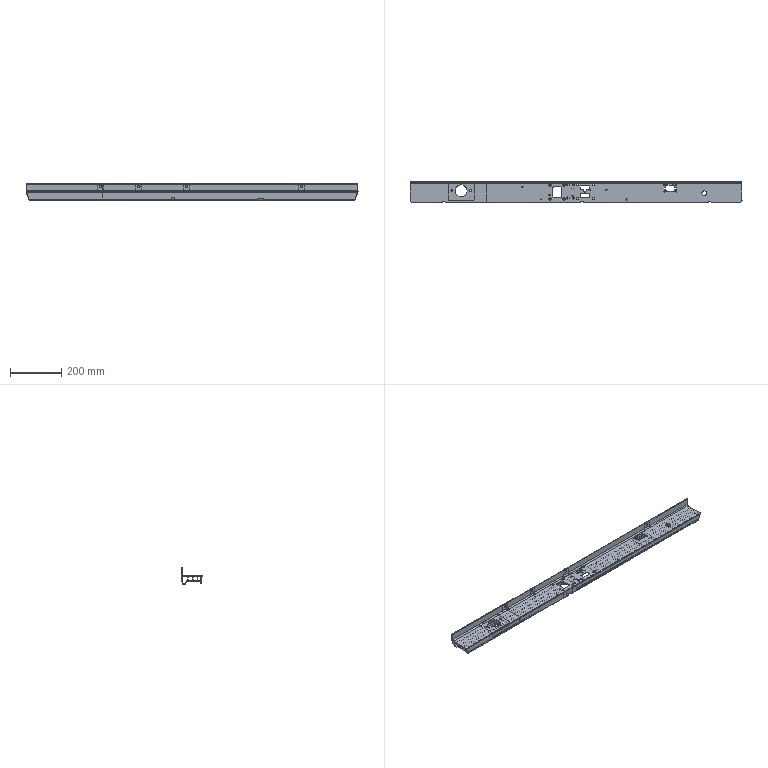NC program | NX | posted with a generic post | part box 1301 x 81.1 x 63 mm
Whole program:
N10 G17 G21 G94 G90
(HOLE_MILLING_1_COPY_2 , TOOL : D6)
N12 T06 M6
N14 G54
N16 G17 G0 G90 X0. Y-10. B0. C0. S6000 M3
N18 G43 Z30. H6
N20 Z0.2
N22 G94 G3 X-0.688 Y-9.313 R0.688 F1400.
N24 X-1.375 Y-10. R0.688
N26 X-1.375 Y-10. Z-0.3 I1.375 J0.
N28 X-1.375 Y-10. Z-0.8 I1.375 J0.
N30 X-1.375 Y-10. Z-1.3 I1.375 J0.
N32 X-1.375 Y-10. Z-1.8 I1.375 J0.
N34 X-1.375 Y-10. Z-2.3 I1.375 J0.
N36 X-1.375 Y-10. Z-2.8 I1.375 J0.
N38 X-1.375 Y-10. Z-3.3 I1.375 J0.
N40 X-1.375 Y-10. Z-3.8 I1.375 J0.
N42 X0. Y-11.375 R1.375
N44 X-1.375 Y-10. R-1.375
N46 X-0.688 Y-10.688 R0.688
N48 X0. Y-10. R0.688
N50 G0 Z30.
N52 X448.999
N54 Z0.2
N56 G3 X448.312 Y-9.313 R0.688
N58 X447.624 Y-10. R0.688
N60 X447.624 Y-10. Z-0.3 I1.375 J0.
N62 X447.624 Y-10. Z-0.8 I1.375 J0.
N64 X447.624 Y-10. Z-1.3 I1.375 J0.
N66 X447.624 Y-10. Z-1.8 I1.375 J0.
N68 X447.624 Y-10. Z-2.3 I1.375 J0.
N70 X447.624 Y-10. Z-2.8 I1.375 J0.
N72 X447.624 Y-10. Z-3.3 I1.375 J0.
N74 X447.624 Y-10. Z-3.8 I1.375 J0.
N76 X448.999 Y-11.375 R1.375
N78 X447.624 Y-10. R-1.375
N80 X448.312 Y-10.688 R0.688
N82 X448.999 Y-10. R0.688
N84 G0 Z30.
N86 X635.999
N88 Z0.2
N90 G3 X635.312 Y-9.313 R0.688
N92 X634.624 Y-10. R0.688
N94 X634.624 Y-10. Z-0.3 I1.375 J0.
N96 X634.624 Y-10. Z-0.8 I1.375 J0.
N98 X634.624 Y-10. Z-1.3 I1.375 J0.
N100 X634.624 Y-10. Z-1.8 I1.375 J0.
N102 X634.624 Y-10. Z-2.3 I1.375 J0.
N104 X634.624 Y-10. Z-2.8 I1.375 J0.
N106 X634.624 Y-10. Z-3.3 I1.375 J0.
N108 X634.624 Y-10. Z-3.8 I1.375 J0.
N110 X635.999 Y-11.375 R1.375
N112 X634.624 Y-10. R-1.375
N114 X635.312 Y-10.688 R0.688
N116 X635.999 Y-10. R0.688
N118 G0 Z30.
N120 X785.999
N122 Z0.2
N124 G3 X785.312 Y-9.313 R0.688
N126 X784.624 Y-10. R0.688
N128 X784.624 Y-10. Z-0.3 I1.375 J0.
N130 X784.624 Y-10. Z-0.8 I1.375 J0.
N132 X784.624 Y-10. Z-1.3 I1.375 J0.
N134 X784.624 Y-10. Z-1.8 I1.375 J0.
N136 X784.624 Y-10. Z-2.3 I1.375 J0.
N138 X784.624 Y-10. Z-2.8 I1.375 J0.
N140 X784.624 Y-10. Z-3.3 I1.375 J0.
N142 X784.624 Y-10. Z-3.8 I1.375 J0.
N144 X785.999 Y-11.375 R1.375
N146 X784.624 Y-10. R-1.375
N148 X785.312 Y-10.688 R0.688
N150 X785.999 Y-10. R0.688
N152 G0 Z30.
N154 M5
(ZLEVEL_PROFILE_COPY_1_COPY_COPY_COPY_COPY_COPY_1 , TOOL : D6A45)
N156 T07 M6
N158 G54
N160 G17 G0 G90 X786.289 Y-8.819 B0. C0. S6000 M3
N162 G43 Z30. H7
N164 Z-2.3
N166 G94 G1 X786.519 Y-7.884 F1000.
N168 G3 X785.999 Y-7.584 R0.6
N170 X783.583 Y-10. R2.416
N172 X785.999 Y-7.584 R-2.416
N174 X785.479 Y-7.884 R0.6
N176 G1 X785.709 Y-8.819
N178 G0 Z30.
N180 X636.289
N182 Z-2.3
N184 G1 X636.519 Y-7.884
N186 G3 X635.999 Y-7.584 R0.6
N188 X633.583 Y-10. R2.416
N190 X635.999 Y-7.584 R-2.416
N192 X635.479 Y-7.884 R0.6
N194 G1 X635.709 Y-8.819
N196 G0 Z30.
N198 X449.289
N200 Z-2.3
N202 G1 X449.519 Y-7.884
N204 G3 X448.999 Y-7.584 R0.6
N206 X446.583 Y-10. R2.416
N208 X448.999 Y-7.584 R-2.416
N210 X448.479 Y-7.884 R0.6
N212 G1 X448.709 Y-8.819
N214 G0 Z30.
N216 X0.29
N218 Z-2.3
N220 G1 X0.52 Y-7.884
N222 G3 X0. Y-7.584 R0.6
N224 X-2.416 Y-10. R2.416
N226 X0. Y-7.584 R-2.416
N228 X-0.52 Y-7.884 R0.6
N230 G1 X-0.29 Y-8.819
N232 G0 Z30.
N234 M5
(刀补16刀补_COPY , TOOL : D6)
N236 T06 M6
N238 G54
N240 G17 G0 G90 X785.999 Y-10. B0. C0. S6000 M3
N242 G43 Z30. H6
N244 Z0.2
N246 G41 G94 G1 X786.002 Y-9.9 F1000. D6
N248 G3 X784.614 Y-10. R0.698
N250 X784.614 Y-10. Z-1.8 I1.385 J0.
N252 X784.614 Y-10. Z-3.8 I1.385 J0.
N254 X785.999 Y-11.385 R1.385
N256 X784.614 Y-10. R-1.385
N258 X786.002 Y-10.1 R0.698
N260 G40
N262 G1 X785.999 Y-10.
N264 G0 Z30.
N266 X635.999
N268 Z0.2
N270 G41 G1 X636.002 Y-9.9
N272 G3 X634.614 Y-10. R0.698
N274 X634.614 Y-10. Z-1.8 I1.385 J0.
N276 X634.614 Y-10. Z-3.8 I1.385 J0.
N278 X635.999 Y-11.385 R1.385
N280 X634.614 Y-10. R-1.385
N282 X636.002 Y-10.1 R0.698
N284 G40
N286 G1 X635.999 Y-10.
N288 G0 Z30.
N290 X448.999
N292 Z0.2
N294 G41 G1 X449.002 Y-9.9
N296 G3 X447.614 Y-10. R0.698
N298 X447.614 Y-10. Z-1.8 I1.385 J0.
N300 X447.614 Y-10. Z-3.8 I1.385 J0.
N302 X448.999 Y-11.385 R1.385
N304 X447.614 Y-10. R-1.385
N306 X449.002 Y-10.1 R0.698
N308 G40
N310 G1 X448.999 Y-10.
N312 G0 Z30.
N314 X0.
N316 Z0.2
N318 G41 G1 X0.003 Y-9.9
N320 G3 X-1.385 Y-10. R0.698
N322 X-1.385 Y-10. Z-1.8 I1.385 J0.
N324 X-1.385 Y-10. Z-3.8 I1.385 J0.
N326 X0. Y-11.385 R1.385
N328 X-1.385 Y-10. R-1.385
N330 X0.003 Y-10.1 R0.698
N332 G40
N334 G1 X0. Y-10.
N336 G0 Z30.
N338 M5
N340 M2